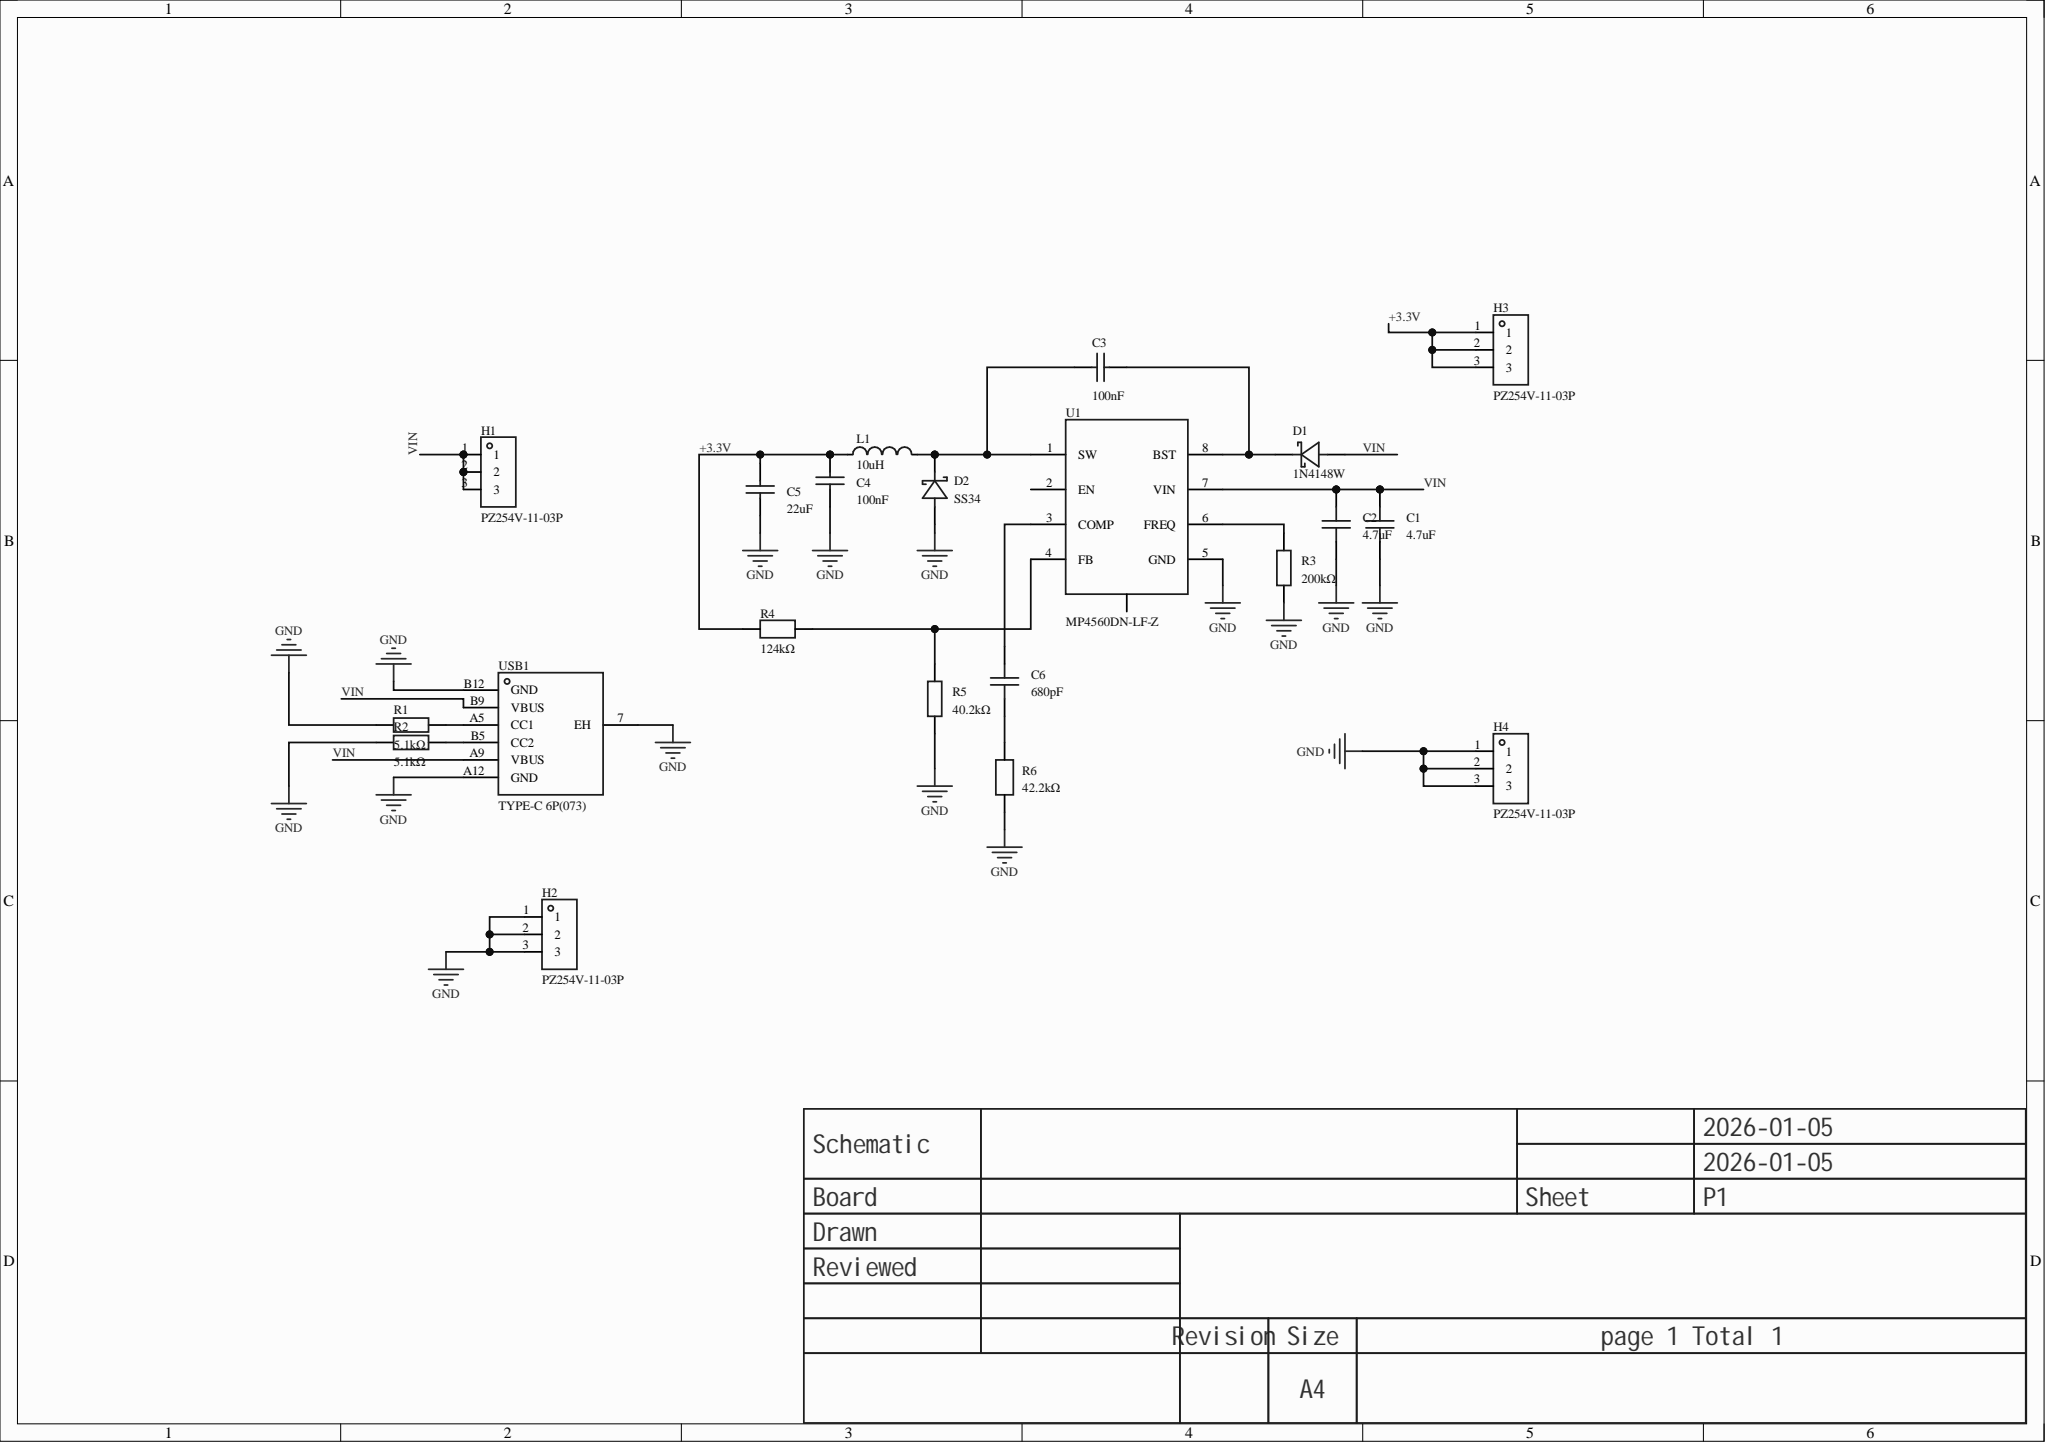Circuit board | Altium Designer | 21 parts | 11 nets
Bill of materials:
Comment,Description,Designator,Footprint,LibRef,Quantity
"4.7uF","Capacitance: 4.7uF; tolerance: ±10%; rated voltage: 100V; temperature coefficient: X7S;","C1, C2","C1206","GRM31CC72A475KE11L","2"
"100nF","Capacitance: 100nF; tolerance: ±10%; rated voltage: 100V; temperature coefficient: X7R;","C3, C4","C0805","CL21B104KCFNNNE","2"
"22uF","Capacitance: 22uF; tolerance: ±10%; rated voltage: 25V; temperature coefficient: X5R;","C5","C1206","CL31A226KAHNNNE","1"
"680pF","Capacitance: 680pF; tolerance: ±5%; rated voltage: 50V; temperature coefficient: C0G;","C6","C0805","CGA0805C0G681J500HT","1"
"1N4148W","Diode configuration: discrete; forward voltage (Vf): 1.25V@150mA; DC reverse voltage (Vr): 100V; rectified current: 150mA; reverse recovery time (Trr): 4ns;","D1","SOD-123_L2.7-W1.6-LS3.7-FD","1N4148W_C7420318","1"
"SS34","Diode configuration: discrete; forward voltage (Vf): 550mV@3.0A; DC reverse voltage (Vr): 40V; rectified current: 3A;","D2","SMA_L4.3-W2.6-LS5.0-FD","SS34_C7420365","1"
"PZ254V-11-03P","Pin structure: 1x3P; pitch: 2.54mm; row spacing: -; round/square pin: square pin; mounting: through-hole; rows: single row; total pins: 3P; rated current: 3A; rated voltage: 250V; mating pin length: 6mm; plastic height: 2.5mm; termination pin length: 3mm; operating temperature: -40℃~+105℃; colour: black;","H1, H2, H3, H4","HDR-TH_3P-P2.54-V-M_PZ254V-11-03P","PZ254V-11-03P","4"
"10uH","Inductance: 10uH; tolerance: ±20%; rated current: 3.2A; saturation current (Isat): 3.5A; type: -;","L1","IND-SMD_L5.2-W5.2_MCW-0530","SMMS0530-100M","1"
"5.1kΩ","Resistor type: thick film resistor; resistance: 5.1kΩ; tolerance: ±1%; power: 125mW; working voltage: 150V; temperature coefficient: ±100ppm/?;","R1, R2","R0805","0805W8F5101T5E","2"
"200kΩ","Resistor type: thick film resistor; resistance: 200kΩ; tolerance: ±1%; power: 125mW; max working voltage: 150V; temperature coefficient: ±100ppm/?;","R3","R0805","0805W8F2003T5E","1"
"124kΩ","Resistor type: thick film resistor; resistance: 124kΩ; tolerance: ±1%; power: 125mW; working voltage: 150V; temperature coefficient: ±100ppm/?;","R4","R0805","FRC0805F1243TS","1"
"40.2kΩ","Resistor type: thick film resistor; resistance: 40.2kΩ; tolerance: ±1%; power: 125mW; working voltage: 150V; temperature coefficient: ±100ppm/?;","R5","R0805","0805W8F4022T5E","1"
"42.2kΩ","Resistor type: thick film resistor; resistance: 42.2kΩ; tolerance: ±1%; power: 125mW; working voltage: 150V; temperature coefficient: ±100ppm/?;","R6","R0805","FRC0805F4222TS","1"
"MP4560DN-LF-Z","Function type: buck; output type: adjustable; working voltage: 3.8V~55V; output voltage: 800mV~52V; output current: 2A;","U1","SOIC-8_L4.9-W3.9-P1.27-LS6.0-BL-EP3.1-1","MP4560DN-LF-Z","1"
"TYPE-C 6P(073)","Connector type: Type-C; standard: USB 3.1; gender: female; mounting: horizontal SMT; contacts: 6P; ports: 1; rated current - power: 3A; operating temperature: -25℃~+85℃;","USB1","TYPE-C-SMD_TYPE-C-6P-073","TYPE-C 6P(073)","1"
Netlist (Protel format):
[
C1
C1206
4.7uF



]
[
C2
C1206
4.7uF



]
[
C3
C0805
100nF



]
[
C4
C0805
100nF



]
[
C5
C1206
22uF



]
[
C6
C0805
680pF



]
[
D1
SOD-123_L2.7-W1.6-LS3.7-FD
1N4148W



]
[
D2
SMA_L4.3-W2.6-LS5.0-FD
SS34



]
[
H1
HDR-TH_3P-P2.54-V-M_PZ254V-11-03P
PZ254V-11-03P



]
[
H2
HDR-TH_3P-P2.54-V-M_PZ254V-11-03P
PZ254V-11-03P



]
[
H3
HDR-TH_3P-P2.54-V-M_PZ254V-11-03P
PZ254V-11-03P



]
[
H4
HDR-TH_3P-P2.54-V-M_PZ254V-11-03P
PZ254V-11-03P



]
[
L1
IND-SMD_L5.2-W5.2_MCW-0530
10uH



]
[
R1
R0805
5.1kΩ



]
[
R2
R0805
5.1kΩ



]
[
R3
R0805
200kΩ



]
[
R4
R0805
124kΩ



]
[
R5
R0805
40.2kΩ



]
[
R6
R0805
42.2kΩ



]
[
U1
SOIC-8_L4.9-W3.9-P1.27-LS6.0-BL-EP3.1-1
MP4560DN-LF-Z



]
[
USB1
TYPE-C-SMD_TYPE-C-6P-073
TYPE-C 6P(073)



]
(
VIN
C1-1
C2-1
D1-1
H1-1
H1-2
H1-3
U1-7
USB1-A9
USB1-B9
)
(
NetR4_2
R4-2
R5-1
U1-4
)
(
NetR3_1
R3-1
U1-6
)
(
NetR2_2
R2-2
USB1-B5
)
(
NetR1_2
R1-2
USB1-A5
)
(
NetC6_2
C6-2
U1-3
)
(
NetC6_1
C6-1
R6-2
)
(
NetC3_2
C3-2
D2-2
L1-2
U1-1
)
(
NetC3_1
C3-1
D1-2
U1-8
)
(
GND
C1-2
C2-2
C4-2
C5-1
D2-1
H2-1
H2-2
H2-3
H4-1
H4-2
H4-3
R1-1
R2-1
R3-2
R5-2
R6-1
U1-5
USB1-7
USB1-A12
USB1-B12
)
(
+3.3V
C4-1
C5-2
H3-1
H3-2
H3-3
L1-1
R4-1
)